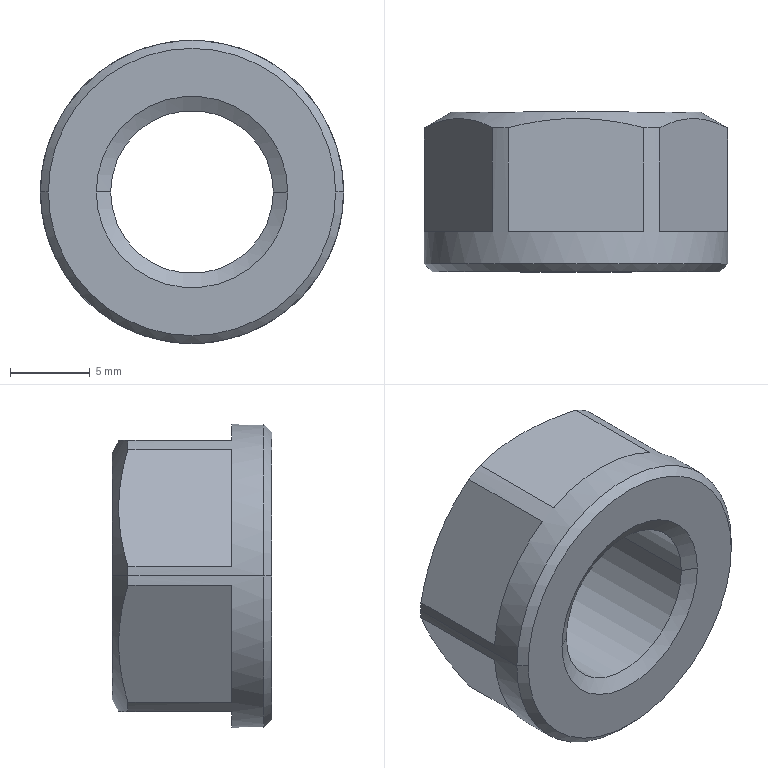Part | SolidWorks | features BaseBody 1 | 1 solid | 26 faces | box 19 x 10 x 19 mm | volume 1716 mm3 | plane 14 | cone 8 | cylinder 4 | commonest cylinder face diameters 10.2 x2 19 x2
STEP:
#1=CARTESIAN_POINT('',(59.5,178.7,-24.25));
#2=VERTEX_POINT('',#1);
#3=CARTESIAN_POINT('',(41.5,178.7,-24.25));
#4=VERTEX_POINT('',#3);
#5=CARTESIAN_POINT('',(50.5,178.7,-24.25));
#6=DIRECTION('',(0.,-1.,0.));
#7=DIRECTION('',(-1.,0.,0.));
#8=AXIS2_PLACEMENT_3D('',#5,#6,#7);
#9=CIRCLE('',#8,9.);
#10=EDGE_CURVE('',#2,#4,#9,.T.);
#11=ORIENTED_EDGE('',*,*,#10,.F.);
#12=CARTESIAN_POINT('',(60.,179.2,-24.25));
#13=VERTEX_POINT('',#12);
#14=CARTESIAN_POINT('',(60.,179.2,-24.25));
#15=DIRECTION('',(0.7071,0.7071,0.));
#16=VECTOR('',#15,1000.);
#17=LINE('',#14,#16);
#18=EDGE_CURVE('',#2,#13,#17,.T.);
#19=ORIENTED_EDGE('',*,*,#18,.T.);
#20=CARTESIAN_POINT('',(41.,179.2,-24.25));
#21=VERTEX_POINT('',#20);
#22=CARTESIAN_POINT('',(50.5,179.2,-24.25));
#23=DIRECTION('',(0.,1.,0.));
#24=DIRECTION('',(-1.,0.,0.));
#25=AXIS2_PLACEMENT_3D('',#22,#23,#24);
#26=CIRCLE('',#25,9.5);
#27=EDGE_CURVE('',#21,#13,#26,.T.);
#28=ORIENTED_EDGE('',*,*,#27,.F.);
#29=CARTESIAN_POINT('',(41.,179.2,-24.25));
#30=DIRECTION('',(-0.7071,0.7071,0.));
#31=VECTOR('',#30,1000.);
#32=LINE('',#29,#31);
#33=EDGE_CURVE('',#4,#21,#32,.T.);
#34=ORIENTED_EDGE('',*,*,#33,.F.);
#35=EDGE_LOOP('',(#11,#19,#28,#34));
#36=FACE_OUTER_BOUND('',#35,.T.);
#37=CARTESIAN_POINT('',(50.5,179.2,-24.25));
#38=DIRECTION('',(0.,1.,0.));
#39=DIRECTION('',(-1.,0.,0.));
#40=AXIS2_PLACEMENT_3D('',#37,#38,#39);
#41=CONICAL_SURFACE('',#40,9.5,0.7854);
#42=ADVANCED_FACE('',(#36),#41,.T.);
#43=CARTESIAN_POINT('',(58.294,188.7,-24.25));
#44=VERTEX_POINT('',#43);
#45=CARTESIAN_POINT('',(42.706,188.7,-24.25));
#46=VERTEX_POINT('',#45);
#47=CARTESIAN_POINT('',(50.5,188.7,-24.25));
#48=DIRECTION('',(0.,1.,0.));
#49=DIRECTION('',(-1.,0.,0.));
#50=AXIS2_PLACEMENT_3D('',#47,#48,#49);
#51=CIRCLE('',#50,7.794);
#52=EDGE_CURVE('',#44,#46,#51,.T.);
#53=ORIENTED_EDGE('',*,*,#52,.F.);
#54=CARTESIAN_POINT('',(60.,187.715,-24.25));
#55=VERTEX_POINT('',#54);
#56=CARTESIAN_POINT('',(58.294,188.7,-24.25));
#57=DIRECTION('',(0.866,-0.5,0.));
#58=VECTOR('',#57,1000.);
#59=LINE('',#56,#58);
#60=EDGE_CURVE('',#44,#55,#59,.T.);
#61=ORIENTED_EDGE('',*,*,#60,.T.);
#62=CARTESIAN_POINT('',(59.983,187.715,-24.826));
#63=VERTEX_POINT('',#62);
#64=CARTESIAN_POINT('',(50.5,187.715,-24.25));
#65=DIRECTION('',(0.,1.,0.));
#66=DIRECTION('',(1.,0.,0.));
#67=AXIS2_PLACEMENT_3D('',#64,#65,#66);
#68=CIRCLE('',#67,9.5);
#69=EDGE_CURVE('',#55,#63,#68,.T.);
#70=ORIENTED_EDGE('',*,*,#69,.T.);
#71=CARTESIAN_POINT('',(55.74,187.715,-32.174));
#72=VERTEX_POINT('',#71);
#73=CARTESIAN_POINT('',(59.983,187.715,-24.826));
#74=CARTESIAN_POINT('',(59.635,187.895,-25.428));
#75=CARTESIAN_POINT('',(59.285,188.039,-26.034));
#76=CARTESIAN_POINT('',(58.581,188.238,-27.254));
#77=CARTESIAN_POINT('',(58.226,188.292,-27.868));
#78=CARTESIAN_POINT('',(57.511,188.293,-29.106));
#79=CARTESIAN_POINT('',(57.15,188.24,-29.732));
#80=CARTESIAN_POINT('',(56.44,188.041,-30.962));
#81=CARTESIAN_POINT('',(56.088,187.895,-31.571));
#82=CARTESIAN_POINT('',(55.74,187.715,-32.174));
#83=B_SPLINE_CURVE_WITH_KNOTS('',3,(#73,#74,#75,#76,#77,#78,#79,#80,#81,#82),.UNSPECIFIED.,.F.,.F.,(4,2,2,2,4),(0.000000295,0.002133,0.004266,0.006398,0.008531),.UNSPECIFIED.);
#84=EDGE_CURVE('',#63,#72,#83,.T.);
#85=ORIENTED_EDGE('',*,*,#84,.T.);
#86=CARTESIAN_POINT('',(54.743,187.715,-32.75));
#87=VERTEX_POINT('',#86);
#88=CARTESIAN_POINT('',(50.5,187.715,-24.25));
#89=DIRECTION('',(0.,1.,0.));
#90=DIRECTION('',(1.,0.,0.));
#91=AXIS2_PLACEMENT_3D('',#88,#89,#90);
#92=CIRCLE('',#91,9.5);
#93=EDGE_CURVE('',#72,#87,#92,.T.);
#94=ORIENTED_EDGE('',*,*,#93,.T.);
#95=CARTESIAN_POINT('',(46.257,187.715,-32.75));
#96=VERTEX_POINT('',#95);
#97=CARTESIAN_POINT('',(54.743,187.715,-32.75));
#98=CARTESIAN_POINT('',(54.047,187.895,-32.75));
#99=CARTESIAN_POINT('',(53.348,188.039,-32.75));
#100=CARTESIAN_POINT('',(51.939,188.238,-32.75));
#101=CARTESIAN_POINT('',(51.23,188.292,-32.75));
#102=CARTESIAN_POINT('',(49.8,188.293,-32.75));
#103=CARTESIAN_POINT('',(49.078,188.24,-32.75));
#104=CARTESIAN_POINT('',(47.657,188.041,-32.75));
#105=CARTESIAN_POINT('',(46.954,187.895,-32.75));
#106=CARTESIAN_POINT('',(46.257,187.715,-32.75));
#107=B_SPLINE_CURVE_WITH_KNOTS('',3,(#97,#98,#99,#100,#101,#102,#103,#104,#105,#106),.UNSPECIFIED.,.F.,.F.,(4,2,2,2,4),(0.000000255,0.002133,0.004266,0.006398,0.008531),.UNSPECIFIED.);
#108=EDGE_CURVE('',#87,#96,#107,.T.);
#109=ORIENTED_EDGE('',*,*,#108,.T.);
#110=CARTESIAN_POINT('',(45.26,187.715,-32.174));
#111=VERTEX_POINT('',#110);
#112=CARTESIAN_POINT('',(50.5,187.715,-24.25));
#113=DIRECTION('',(0.,1.,0.));
#114=DIRECTION('',(1.,0.,0.));
#115=AXIS2_PLACEMENT_3D('',#112,#113,#114);
#116=CIRCLE('',#115,9.5);
#117=EDGE_CURVE('',#96,#111,#116,.T.);
#118=ORIENTED_EDGE('',*,*,#117,.T.);
#119=CARTESIAN_POINT('',(41.017,187.715,-24.826));
#120=VERTEX_POINT('',#119);
#121=CARTESIAN_POINT('',(45.26,187.715,-32.174));
#122=CARTESIAN_POINT('',(44.912,187.895,-31.572));
#123=CARTESIAN_POINT('',(44.563,188.039,-30.966));
#124=CARTESIAN_POINT('',(43.858,188.238,-29.746));
#125=CARTESIAN_POINT('',(43.504,188.292,-29.132));
#126=CARTESIAN_POINT('',(42.789,188.293,-27.894));
#127=CARTESIAN_POINT('',(42.428,188.24,-27.268));
#128=CARTESIAN_POINT('',(41.717,188.041,-26.038));
#129=CARTESIAN_POINT('',(41.366,187.895,-25.429));
#130=CARTESIAN_POINT('',(41.017,187.715,-24.826));
#131=B_SPLINE_CURVE_WITH_KNOTS('',3,(#121,#122,#123,#124,#125,#126,#127,#128,#129,#130),.UNSPECIFIED.,.F.,.F.,(4,2,2,2,4),(0.000000295,0.002133,0.004266,0.006398,0.008531),.UNSPECIFIED.);
#132=EDGE_CURVE('',#111,#120,#131,.T.);
#133=ORIENTED_EDGE('',*,*,#132,.T.);
#134=CARTESIAN_POINT('',(41.,187.715,-24.25));
#135=VERTEX_POINT('',#134);
#136=CARTESIAN_POINT('',(50.5,187.715,-24.25));
#137=DIRECTION('',(0.,1.,0.));
#138=DIRECTION('',(1.,0.,0.));
#139=AXIS2_PLACEMENT_3D('',#136,#137,#138);
#140=CIRCLE('',#139,9.5);
#141=EDGE_CURVE('',#120,#135,#140,.T.);
#142=ORIENTED_EDGE('',*,*,#141,.T.);
#143=CARTESIAN_POINT('',(42.706,188.7,-24.25));
#144=DIRECTION('',(-0.866,-0.5,0.));
#145=VECTOR('',#144,1000.);
#146=LINE('',#143,#145);
#147=EDGE_CURVE('',#46,#135,#146,.T.);
#148=ORIENTED_EDGE('',*,*,#147,.F.);
#149=EDGE_LOOP('',(#53,#61,#70,#85,#94,#109,#118,#133,#142,#148));
#150=FACE_OUTER_BOUND('',#149,.T.);
#151=CARTESIAN_POINT('',(50.5,188.7,-24.25));
#152=DIRECTION('',(0.,-1.,0.));
#153=DIRECTION('',(-1.,0.,0.));
#154=AXIS2_PLACEMENT_3D('',#151,#152,#153);
#155=CONICAL_SURFACE('',#154,7.794,1.047);
#156=ADVANCED_FACE('',(#150),#155,.T.);
#157=CARTESIAN_POINT('',(55.6,179.22,-24.25));
#158=VERTEX_POINT('',#157);
#159=CARTESIAN_POINT('',(45.4,179.22,-24.25));
#160=VERTEX_POINT('',#159);
#161=CARTESIAN_POINT('',(50.5,179.22,-24.25));
#162=DIRECTION('',(0.,1.,0.));
#163=DIRECTION('',(-1.,0.,0.));
#164=AXIS2_PLACEMENT_3D('',#161,#162,#163);
#165=CIRCLE('',#164,5.1);
#166=EDGE_CURVE('',#158,#160,#165,.T.);
#167=ORIENTED_EDGE('',*,*,#166,.T.);
#168=CARTESIAN_POINT('',(44.5,178.7,-24.25));
#169=VERTEX_POINT('',#168);
#170=CARTESIAN_POINT('',(45.4,179.22,-24.25));
#171=DIRECTION('',(-0.866,-0.5,0.));
#172=VECTOR('',#171,1000.);
#173=LINE('',#170,#172);
#174=EDGE_CURVE('',#160,#169,#173,.T.);
#175=ORIENTED_EDGE('',*,*,#174,.T.);
#176=CARTESIAN_POINT('',(56.5,178.7,-24.25));
#177=VERTEX_POINT('',#176);
#178=CARTESIAN_POINT('',(50.5,178.7,-24.25));
#179=DIRECTION('',(0.,1.,0.));
#180=DIRECTION('',(-1.,0.,0.));
#181=AXIS2_PLACEMENT_3D('',#178,#179,#180);
#182=CIRCLE('',#181,6.);
#183=EDGE_CURVE('',#177,#169,#182,.T.);
#184=ORIENTED_EDGE('',*,*,#183,.F.);
#185=CARTESIAN_POINT('',(55.6,179.22,-24.25));
#186=DIRECTION('',(0.866,-0.5,0.));
#187=VECTOR('',#186,1000.);
#188=LINE('',#185,#187);
#189=EDGE_CURVE('',#158,#177,#188,.T.);
#190=ORIENTED_EDGE('',*,*,#189,.F.);
#191=EDGE_LOOP('',(#167,#175,#184,#190));
#192=FACE_OUTER_BOUND('',#191,.T.);
#193=CARTESIAN_POINT('',(50.5,179.22,-24.25));
#194=DIRECTION('',(0.,-1.,0.));
#195=DIRECTION('',(1.,0.,0.));
#196=AXIS2_PLACEMENT_3D('',#193,#194,#195);
#197=CONICAL_SURFACE('',#196,5.1,1.047);
#198=ADVANCED_FACE('',(#192),#197,.F.);
#199=ORIENTED_EDGE('',*,*,#166,.F.);
#200=CARTESIAN_POINT('',(55.6,188.18,-24.25));
#201=VERTEX_POINT('',#200);
#202=CARTESIAN_POINT('',(55.6,188.7,-24.25));
#203=DIRECTION('',(0.,1.,0.));
#204=VECTOR('',#203,1000.);
#205=LINE('',#202,#204);
#206=EDGE_CURVE('',#158,#201,#205,.T.);
#207=ORIENTED_EDGE('',*,*,#206,.T.);
#208=CARTESIAN_POINT('',(45.4,188.18,-24.25));
#209=VERTEX_POINT('',#208);
#210=CARTESIAN_POINT('',(50.5,188.18,-24.25));
#211=DIRECTION('',(0.,1.,0.));
#212=DIRECTION('',(-1.,0.,0.));
#213=AXIS2_PLACEMENT_3D('',#210,#211,#212);
#214=CIRCLE('',#213,5.1);
#215=EDGE_CURVE('',#201,#209,#214,.T.);
#216=ORIENTED_EDGE('',*,*,#215,.T.);
#217=CARTESIAN_POINT('',(45.4,188.7,-24.25));
#218=DIRECTION('',(0.,1.,0.));
#219=VECTOR('',#218,1000.);
#220=LINE('',#217,#219);
#221=EDGE_CURVE('',#160,#209,#220,.T.);
#222=ORIENTED_EDGE('',*,*,#221,.F.);
#223=EDGE_LOOP('',(#199,#207,#216,#222));
#224=FACE_OUTER_BOUND('',#223,.T.);
#225=CARTESIAN_POINT('',(50.5,188.7,-24.25));
#226=DIRECTION('',(0.,1.,0.));
#227=DIRECTION('',(-1.,0.,0.));
#228=AXIS2_PLACEMENT_3D('',#225,#226,#227);
#229=CYLINDRICAL_SURFACE('',#228,5.1);
#230=ADVANCED_FACE('',(#224),#229,.F.);
#231=ORIENTED_EDGE('',*,*,#215,.F.);
#232=CARTESIAN_POINT('',(56.5,188.7,-24.25));
#233=VERTEX_POINT('',#232);
#234=CARTESIAN_POINT('',(56.5,188.7,-24.25));
#235=DIRECTION('',(0.866,0.5,0.));
#236=VECTOR('',#235,1000.);
#237=LINE('',#234,#236);
#238=EDGE_CURVE('',#201,#233,#237,.T.);
#239=ORIENTED_EDGE('',*,*,#238,.T.);
#240=CARTESIAN_POINT('',(44.5,188.7,-24.25));
#241=VERTEX_POINT('',#240);
#242=CARTESIAN_POINT('',(50.5,188.7,-24.25));
#243=DIRECTION('',(0.,1.,0.));
#244=DIRECTION('',(-1.,0.,0.));
#245=AXIS2_PLACEMENT_3D('',#242,#243,#244);
#246=CIRCLE('',#245,6.);
#247=EDGE_CURVE('',#233,#241,#246,.T.);
#248=ORIENTED_EDGE('',*,*,#247,.T.);
#249=CARTESIAN_POINT('',(44.5,188.7,-24.25));
#250=DIRECTION('',(-0.866,0.5,0.));
#251=VECTOR('',#250,1000.);
#252=LINE('',#249,#251);
#253=EDGE_CURVE('',#209,#241,#252,.T.);
#254=ORIENTED_EDGE('',*,*,#253,.F.);
#255=EDGE_LOOP('',(#231,#239,#248,#254));
#256=FACE_OUTER_BOUND('',#255,.T.);
#257=CARTESIAN_POINT('',(50.5,188.7,-24.25));
#258=DIRECTION('',(0.,1.,0.));
#259=DIRECTION('',(-1.,0.,0.));
#260=AXIS2_PLACEMENT_3D('',#257,#258,#259);
#261=CONICAL_SURFACE('',#260,6.,1.047);
#262=ADVANCED_FACE('',(#256),#261,.F.);
#263=CARTESIAN_POINT('',(41.017,187.715,-23.674));
#264=VERTEX_POINT('',#263);
#265=CARTESIAN_POINT('',(50.5,187.715,-24.25));
#266=DIRECTION('',(0.,1.,0.));
#267=DIRECTION('',(1.,0.,0.));
#268=AXIS2_PLACEMENT_3D('',#265,#266,#267);
#269=CIRCLE('',#268,9.5);
#270=EDGE_CURVE('',#135,#264,#269,.T.);
#271=ORIENTED_EDGE('',*,*,#270,.F.);
#272=CARTESIAN_POINT('',(41.,181.2,-24.25));
#273=DIRECTION('',(0.,-1.,0.));
#274=VECTOR('',#273,1000.);
#275=LINE('',#272,#274);
#276=EDGE_CURVE('',#135,#21,#275,.T.);
#277=ORIENTED_EDGE('',*,*,#276,.T.);
#278=ORIENTED_EDGE('',*,*,#27,.T.);
#279=CARTESIAN_POINT('',(60.,181.2,-24.25));
#280=DIRECTION('',(0.,-1.,0.));
#281=VECTOR('',#280,1000.);
#282=LINE('',#279,#281);
#283=EDGE_CURVE('',#55,#13,#282,.T.);
#284=ORIENTED_EDGE('',*,*,#283,.F.);
#285=CARTESIAN_POINT('',(59.983,187.715,-23.674));
#286=VERTEX_POINT('',#285);
#287=CARTESIAN_POINT('',(50.5,187.715,-24.25));
#288=DIRECTION('',(0.,1.,0.));
#289=DIRECTION('',(1.,0.,0.));
#290=AXIS2_PLACEMENT_3D('',#287,#288,#289);
#291=CIRCLE('',#290,9.5);
#292=EDGE_CURVE('',#286,#55,#291,.T.);
#293=ORIENTED_EDGE('',*,*,#292,.F.);
#294=CARTESIAN_POINT('',(59.983,181.2,-23.674));
#295=VERTEX_POINT('',#294);
#296=CARTESIAN_POINT('',(59.983,224.195,-23.674));
#297=DIRECTION('',(0.,-1.,0.));
#298=VECTOR('',#297,1000.);
#299=LINE('',#296,#298);
#300=EDGE_CURVE('',#286,#295,#299,.T.);
#301=ORIENTED_EDGE('',*,*,#300,.T.);
#302=CARTESIAN_POINT('',(55.74,181.2,-16.326));
#303=VERTEX_POINT('',#302);
#304=CARTESIAN_POINT('',(50.5,181.2,-24.25));
#305=DIRECTION('',(0.,1.,0.));
#306=DIRECTION('',(-1.,0.,0.));
#307=AXIS2_PLACEMENT_3D('',#304,#305,#306);
#308=CIRCLE('',#307,9.5);
#309=EDGE_CURVE('',#303,#295,#308,.T.);
#310=ORIENTED_EDGE('',*,*,#309,.F.);
#311=CARTESIAN_POINT('',(55.74,187.715,-16.326));
#312=VERTEX_POINT('',#311);
#313=CARTESIAN_POINT('',(55.74,224.195,-16.326));
#314=DIRECTION('',(0.,-1.,0.));
#315=VECTOR('',#314,1000.);
#316=LINE('',#313,#315);
#317=EDGE_CURVE('',#312,#303,#316,.T.);
#318=ORIENTED_EDGE('',*,*,#317,.F.);
#319=CARTESIAN_POINT('',(54.743,187.715,-15.75));
#320=VERTEX_POINT('',#319);
#321=CARTESIAN_POINT('',(50.5,187.715,-24.25));
#322=DIRECTION('',(0.,1.,0.));
#323=DIRECTION('',(1.,0.,0.));
#324=AXIS2_PLACEMENT_3D('',#321,#322,#323);
#325=CIRCLE('',#324,9.5);
#326=EDGE_CURVE('',#320,#312,#325,.T.);
#327=ORIENTED_EDGE('',*,*,#326,.F.);
#328=CARTESIAN_POINT('',(54.743,181.2,-15.75));
#329=VERTEX_POINT('',#328);
#330=CARTESIAN_POINT('',(54.743,224.195,-15.75));
#331=DIRECTION('',(0.,-1.,0.));
#332=VECTOR('',#331,1000.);
#333=LINE('',#330,#332);
#334=EDGE_CURVE('',#320,#329,#333,.T.);
#335=ORIENTED_EDGE('',*,*,#334,.T.);
#336=CARTESIAN_POINT('',(46.257,181.2,-15.75));
#337=VERTEX_POINT('',#336);
#338=CARTESIAN_POINT('',(50.5,181.2,-24.25));
#339=DIRECTION('',(0.,1.,0.));
#340=DIRECTION('',(-1.,0.,0.));
#341=AXIS2_PLACEMENT_3D('',#338,#339,#340);
#342=CIRCLE('',#341,9.5);
#343=EDGE_CURVE('',#337,#329,#342,.T.);
#344=ORIENTED_EDGE('',*,*,#343,.F.);
#345=CARTESIAN_POINT('',(46.257,187.715,-15.75));
#346=VERTEX_POINT('',#345);
#347=CARTESIAN_POINT('',(46.257,224.195,-15.75));
#348=DIRECTION('',(0.,-1.,0.));
#349=VECTOR('',#348,1000.);
#350=LINE('',#347,#349);
#351=EDGE_CURVE('',#346,#337,#350,.T.);
#352=ORIENTED_EDGE('',*,*,#351,.F.);
#353=CARTESIAN_POINT('',(45.26,187.715,-16.326));
#354=VERTEX_POINT('',#353);
#355=CARTESIAN_POINT('',(50.5,187.715,-24.25));
#356=DIRECTION('',(0.,1.,0.));
#357=DIRECTION('',(1.,0.,0.));
#358=AXIS2_PLACEMENT_3D('',#355,#356,#357);
#359=CIRCLE('',#358,9.5);
#360=EDGE_CURVE('',#354,#346,#359,.T.);
#361=ORIENTED_EDGE('',*,*,#360,.F.);
#362=CARTESIAN_POINT('',(45.26,181.2,-16.326));
#363=VERTEX_POINT('',#362);
#364=CARTESIAN_POINT('',(45.26,224.195,-16.326));
#365=DIRECTION('',(0.,-1.,0.));
#366=VECTOR('',#365,1000.);
#367=LINE('',#364,#366);
#368=EDGE_CURVE('',#354,#363,#367,.T.);
#369=ORIENTED_EDGE('',*,*,#368,.T.);
#370=CARTESIAN_POINT('',(41.017,181.2,-23.674));
#371=VERTEX_POINT('',#370);
#372=CARTESIAN_POINT('',(50.5,181.2,-24.25));
#373=DIRECTION('',(0.,1.,0.));
#374=DIRECTION('',(-1.,0.,0.));
#375=AXIS2_PLACEMENT_3D('',#372,#373,#374);
#376=CIRCLE('',#375,9.5);
#377=EDGE_CURVE('',#371,#363,#376,.T.);
#378=ORIENTED_EDGE('',*,*,#377,.F.);
#379=CARTESIAN_POINT('',(41.017,224.195,-23.674));
#380=DIRECTION('',(0.,-1.,0.));
#381=VECTOR('',#380,1000.);
#382=LINE('',#379,#381);
#383=EDGE_CURVE('',#264,#371,#382,.T.);
#384=ORIENTED_EDGE('',*,*,#383,.F.);
#385=EDGE_LOOP('',(#271,#277,#278,#284,#293,#301,#310,#318,#327,#335,#344,#352,#361,#369,#378,#384));
#386=FACE_OUTER_BOUND('',#385,.T.);
#387=CARTESIAN_POINT('',(50.5,181.2,-24.25));
#388=DIRECTION('',(0.,-1.,0.));
#389=DIRECTION('',(1.,0.,0.));
#390=AXIS2_PLACEMENT_3D('',#387,#388,#389);
#391=CYLINDRICAL_SURFACE('',#390,9.5);
#392=ADVANCED_FACE('',(#386),#391,.T.);
#393=ORIENTED_EDGE('',*,*,#276,.F.);
#394=ORIENTED_EDGE('',*,*,#141,.F.);
#395=CARTESIAN_POINT('',(41.017,181.2,-24.826));
#396=VERTEX_POINT('',#395);
#397=CARTESIAN_POINT('',(41.017,224.195,-24.826));
#398=DIRECTION('',(0.,-1.,0.));
#399=VECTOR('',#398,1000.);
#400=LINE('',#397,#399);
#401=EDGE_CURVE('',#120,#396,#400,.T.);
#402=ORIENTED_EDGE('',*,*,#401,.T.);
#403=CARTESIAN_POINT('',(45.26,181.2,-32.174));
#404=VERTEX_POINT('',#403);
#405=CARTESIAN_POINT('',(50.5,181.2,-24.25));
#406=DIRECTION('',(0.,1.,0.));
#407=DIRECTION('',(-1.,0.,0.));
#408=AXIS2_PLACEMENT_3D('',#405,#406,#407);
#409=CIRCLE('',#408,9.5);
#410=EDGE_CURVE('',#404,#396,#409,.T.);
#411=ORIENTED_EDGE('',*,*,#410,.F.);
#412=CARTESIAN_POINT('',(45.26,224.195,-32.174));
#413=DIRECTION('',(0.,-1.,0.));
#414=VECTOR('',#413,1000.);
#415=LINE('',#412,#414);
#416=EDGE_CURVE('',#111,#404,#415,.T.);
#417=ORIENTED_EDGE('',*,*,#416,.F.);
#418=ORIENTED_EDGE('',*,*,#117,.F.);
#419=CARTESIAN_POINT('',(46.257,181.2,-32.75));
#420=VERTEX_POINT('',#419);
#421=CARTESIAN_POINT('',(46.257,224.195,-32.75));
#422=DIRECTION('',(0.,-1.,0.));
#423=VECTOR('',#422,1000.);
#424=LINE('',#421,#423);
#425=EDGE_CURVE('',#96,#420,#424,.T.);
#426=ORIENTED_EDGE('',*,*,#425,.T.);
#427=CARTESIAN_POINT('',(54.743,181.2,-32.75));
#428=VERTEX_POINT('',#427);
#429=CARTESIAN_POINT('',(50.5,181.2,-24.25));
#430=DIRECTION('',(0.,1.,0.));
#431=DIRECTION('',(-1.,0.,0.));
#432=AXIS2_PLACEMENT_3D('',#429,#430,#431);
#433=CIRCLE('',#432,9.5);
#434=EDGE_CURVE('',#428,#420,#433,.T.);
#435=ORIENTED_EDGE('',*,*,#434,.F.);
#436=CARTESIAN_POINT('',(54.743,224.195,-32.75));
#437=DIRECTION('',(0.,-1.,0.));
#438=VECTOR('',#437,1000.);
#439=LINE('',#436,#438);
#440=EDGE_CURVE('',#87,#428,#439,.T.);
#441=ORIENTED_EDGE('',*,*,#440,.F.);
#442=ORIENTED_EDGE('',*,*,#93,.F.);
#443=CARTESIAN_POINT('',(55.74,181.2,-32.174));
#444=VERTEX_POINT('',#443);
#445=CARTESIAN_POINT('',(55.74,224.195,-32.174));
#446=DIRECTION('',(0.,-1.,0.));
#447=VECTOR('',#446,1000.);
#448=LINE('',#445,#447);
#449=EDGE_CURVE('',#72,#444,#448,.T.);
#450=ORIENTED_EDGE('',*,*,#449,.T.);
#451=CARTESIAN_POINT('',(59.983,181.2,-24.826));
#452=VERTEX_POINT('',#451);
#453=CARTESIAN_POINT('',(50.5,181.2,-24.25));
#454=DIRECTION('',(0.,1.,0.));
#455=DIRECTION('',(-1.,0.,0.));
#456=AXIS2_PLACEMENT_3D('',#453,#454,#455);
#457=CIRCLE('',#456,9.5);
#458=EDGE_CURVE('',#452,#444,#457,.T.);
#459=ORIENTED_EDGE('',*,*,#458,.F.);
#460=CARTESIAN_POINT('',(59.983,224.195,-24.826));
#461=DIRECTION('',(0.,-1.,0.));
#462=VECTOR('',#461,1000.);
#463=LINE('',#460,#462);
#464=EDGE_CURVE('',#63,#452,#463,.T.);
#465=ORIENTED_EDGE('',*,*,#464,.F.);
#466=ORIENTED_EDGE('',*,*,#69,.F.);
#467=ORIENTED_EDGE('',*,*,#283,.T.);
#468=CARTESIAN_POINT('',(50.5,179.2,-24.25));
#469=DIRECTION('',(0.,1.,0.));
#470=DIRECTION('',(-1.,0.,0.));
#471=AXIS2_PLACEMENT_3D('',#468,#469,#470);
#472=CIRCLE('',#471,9.5);
#473=EDGE_CURVE('',#13,#21,#472,.T.);
#474=ORIENTED_EDGE('',*,*,#473,.T.);
#475=EDGE_LOOP('',(#393,#394,#402,#411,#417,#418,#426,#435,#441,#442,#450,#459,#465,#466,#467,#474));
#476=FACE_OUTER_BOUND('',#475,.T.);
#477=CARTESIAN_POINT('',(50.5,181.2,-24.25));
#478=DIRECTION('',(0.,-1.,0.));
#479=DIRECTION('',(1.,0.,0.));
#480=AXIS2_PLACEMENT_3D('',#477,#478,#479);
#481=CYLINDRICAL_SURFACE('',#480,9.5);
#482=ADVANCED_FACE('',(#476),#481,.T.);
#483=CARTESIAN_POINT('',(46.257,187.715,-15.75));
#484=CARTESIAN_POINT('',(46.953,187.895,-15.75));
#485=CARTESIAN_POINT('',(47.652,188.039,-15.75));
#486=CARTESIAN_POINT('',(49.061,188.238,-15.75));
#487=CARTESIAN_POINT('',(49.77,188.292,-15.75));
#488=CARTESIAN_POINT('',(51.2,188.293,-15.75));
#489=CARTESIAN_POINT('',(51.922,188.24,-15.75));
#490=CARTESIAN_POINT('',(53.343,188.041,-15.75));
#491=CARTESIAN_POINT('',(54.046,187.895,-15.75));
#492=CARTESIAN_POINT('',(54.743,187.715,-15.75));
#493=B_SPLINE_CURVE_WITH_KNOTS('',3,(#483,#484,#485,#486,#487,#488,#489,#490,#491,#492),.UNSPECIFIED.,.F.,.F.,(4,2,2,2,4),(0.000000255,0.002133,0.004266,0.006398,0.008531),.UNSPECIFIED.);
#494=EDGE_CURVE('',#346,#320,#493,.T.);
#495=ORIENTED_EDGE('',*,*,#494,.F.);
#496=ORIENTED_EDGE('',*,*,#351,.T.);
#497=CARTESIAN_POINT('',(46.257,181.2,-15.75));
#498=DIRECTION('',(1.,0.,0.));
#499=VECTOR('',#498,1000.);
#500=LINE('',#497,#499);
#501=EDGE_CURVE('',#337,#329,#500,.T.);
#502=ORIENTED_EDGE('',*,*,#501,.T.);
#503=ORIENTED_EDGE('',*,*,#334,.F.);
#504=EDGE_LOOP('',(#495,#496,#502,#503));
#505=FACE_OUTER_BOUND('',#504,.T.);
#506=CARTESIAN_POINT('',(46.257,224.195,-15.75));
#507=DIRECTION('',(0.,0.,-1.));
#508=DIRECTION('',(0.,-1.,0.));
#509=AXIS2_PLACEMENT_3D('',#506,#507,#508);
#510=PLANE('',#509);
#511=ADVANCED_FACE('',(#505),#510,.F.);
#512=CARTESIAN_POINT('',(55.74,187.715,-16.326));
#513=CARTESIAN_POINT('',(56.088,187.895,-16.928));
#514=CARTESIAN_POINT('',(56.437,188.039,-17.534));
#515=CARTESIAN_POINT('',(57.142,188.238,-18.754));
#516=CARTESIAN_POINT('',(57.496,188.292,-19.368));
#517=CARTESIAN_POINT('',(58.211,188.293,-20.606));
#518=CARTESIAN_POINT('',(58.572,188.24,-21.232));
#519=CARTESIAN_POINT('',(59.283,188.041,-22.462));
#520=CARTESIAN_POINT('',(59.634,187.895,-23.071));
#521=CARTESIAN_POINT('',(59.983,187.715,-23.674));
#522=B_SPLINE_CURVE_WITH_KNOTS('',3,(#512,#513,#514,#515,#516,#517,#518,#519,#520,#521),.UNSPECIFIED.,.F.,.F.,(4,2,2,2,4),(0.000000295,0.002133,0.004266,0.006398,0.008531),.UNSPECIFIED.);
#523=EDGE_CURVE('',#312,#286,#522,.T.);
#524=ORIENTED_EDGE('',*,*,#523,.F.);
#525=ORIENTED_EDGE('',*,*,#317,.T.);
#526=CARTESIAN_POINT('',(55.74,181.2,-16.326));
#527=DIRECTION('',(0.5,0.,-0.866));
#528=VECTOR('',#527,1000.);
#529=LINE('',#526,#528);
#530=EDGE_CURVE('',#303,#295,#529,.T.);
#531=ORIENTED_EDGE('',*,*,#530,.T.);
#532=ORIENTED_EDGE('',*,*,#300,.F.);
#533=EDGE_LOOP('',(#524,#525,#531,#532));
#534=FACE_OUTER_BOUND('',#533,.T.);
#535=CARTESIAN_POINT('',(55.74,224.195,-16.326));
#536=DIRECTION('',(-0.866,0.,-0.5));
#537=DIRECTION('',(-0.5,0.,0.866));
#538=AXIS2_PLACEMENT_3D('',#535,#536,#537);
#539=PLANE('',#538);
#540=ADVANCED_FACE('',(#534),#539,.F.);
#541=ORIENTED_EDGE('',*,*,#84,.F.);
#542=ORIENTED_EDGE('',*,*,#464,.T.);
#543=CARTESIAN_POINT('',(59.983,181.2,-24.826));
#544=DIRECTION('',(-0.5,0.,-0.866));
#545=VECTOR('',#544,1000.);
#546=LINE('',#543,#545);
#547=EDGE_CURVE('',#452,#444,#546,.T.);
#548=ORIENTED_EDGE('',*,*,#547,.T.);
#549=ORIENTED_EDGE('',*,*,#449,.F.);
#550=EDGE_LOOP('',(#541,#542,#548,#549));
#551=FACE_OUTER_BOUND('',#550,.T.);
#552=CARTESIAN_POINT('',(59.983,224.195,-24.826));
#553=DIRECTION('',(-0.866,0.,0.5));
#554=DIRECTION('',(0.5,0.,0.866));
#555=AXIS2_PLACEMENT_3D('',#552,#553,#554);
#556=PLANE('',#555);
#557=ADVANCED_FACE('',(#551),#556,.F.);
#558=ORIENTED_EDGE('',*,*,#108,.F.);
#559=ORIENTED_EDGE('',*,*,#440,.T.);
#560=CARTESIAN_POINT('',(54.743,181.2,-32.75));
#561=DIRECTION('',(-1.,0.,0.));
#562=VECTOR('',#561,1000.);
#563=LINE('',#560,#562);
#564=EDGE_CURVE('',#428,#420,#563,.T.);
#565=ORIENTED_EDGE('',*,*,#564,.T.);
#566=ORIENTED_EDGE('',*,*,#425,.F.);
#567=EDGE_LOOP('',(#558,#559,#565,#566));
#568=FACE_OUTER_BOUND('',#567,.T.);
#569=CARTESIAN_POINT('',(54.743,224.195,-32.75));
#570=DIRECTION('',(0.,0.,1.));
#571=DIRECTION('',(0.,1.,0.));
#572=AXIS2_PLACEMENT_3D('',#569,#570,#571);
#573=PLANE('',#572);
#574=ADVANCED_FACE('',(#568),#573,.F.);
#575=ORIENTED_EDGE('',*,*,#132,.F.);
#576=ORIENTED_EDGE('',*,*,#416,.T.);
#577=CARTESIAN_POINT('',(45.26,181.2,-32.174));
#578=DIRECTION('',(-0.5,0.,0.866));
#579=VECTOR('',#578,1000.);
#580=LINE('',#577,#579);
#581=EDGE_CURVE('',#404,#396,#580,.T.);
#582=ORIENTED_EDGE('',*,*,#581,.T.);
#583=ORIENTED_EDGE('',*,*,#401,.F.);
#584=EDGE_LOOP('',(#575,#576,#582,#583));
#585=FACE_OUTER_BOUND('',#584,.T.);
#586=CARTESIAN_POINT('',(45.26,224.195,-32.174));
#587=DIRECTION('',(0.866,0.,0.5));
#588=DIRECTION('',(0.5,0.,-0.866));
#589=AXIS2_PLACEMENT_3D('',#586,#587,#588);
#590=PLANE('',#589);
#591=ADVANCED_FACE('',(#585),#590,.F.);
#592=CARTESIAN_POINT('',(41.017,187.715,-23.674));
#593=CARTESIAN_POINT('',(41.365,187.895,-23.072));
#594=CARTESIAN_POINT('',(41.715,188.039,-22.466));
#595=CARTESIAN_POINT('',(42.419,188.238,-21.246));
#596=CARTESIAN_POINT('',(42.774,188.292,-20.632));
#597=CARTESIAN_POINT('',(43.489,188.293,-19.394));
#598=CARTESIAN_POINT('',(43.85,188.24,-18.768));
#599=CARTESIAN_POINT('',(44.56,188.041,-17.538));
#600=CARTESIAN_POINT('',(44.912,187.895,-16.929));
#601=CARTESIAN_POINT('',(45.26,187.715,-16.326));
#602=B_SPLINE_CURVE_WITH_KNOTS('',3,(#592,#593,#594,#595,#596,#597,#598,#599,#600,#601),.UNSPECIFIED.,.F.,.F.,(4,2,2,2,4),(0.000000295,0.002133,0.004266,0.006398,0.008531),.UNSPECIFIED.);
#603=EDGE_CURVE('',#264,#354,#602,.T.);
#604=ORIENTED_EDGE('',*,*,#603,.F.);
#605=ORIENTED_EDGE('',*,*,#383,.T.);
#606=CARTESIAN_POINT('',(41.017,181.2,-23.674));
#607=DIRECTION('',(0.5,0.,0.866));
#608=VECTOR('',#607,1000.);
#609=LINE('',#606,#608);
#610=EDGE_CURVE('',#371,#363,#609,.T.);
#611=ORIENTED_EDGE('',*,*,#610,.T.);
#612=ORIENTED_EDGE('',*,*,#368,.F.);
#613=EDGE_LOOP('',(#604,#605,#611,#612));
#614=FACE_OUTER_BOUND('',#613,.T.);
#615=CARTESIAN_POINT('',(41.017,224.195,-23.674));
#616=DIRECTION('',(0.866,0.,-0.5));
#617=DIRECTION('',(-0.5,0.,-0.866));
#618=AXIS2_PLACEMENT_3D('',#615,#616,#617);
#619=PLANE('',#618);
#620=ADVANCED_FACE('',(#614),#619,.F.);
#621=CARTESIAN_POINT('',(50.5,188.7,-24.25));
#622=DIRECTION('',(0.,1.,0.));
#623=DIRECTION('',(-1.,0.,0.));
#624=AXIS2_PLACEMENT_3D('',#621,#622,#623);
#625=CIRCLE('',#624,6.);
#626=EDGE_CURVE('',#241,#233,#625,.T.);
#627=ORIENTED_EDGE('',*,*,#626,.F.);
#628=ORIENTED_EDGE('',*,*,#247,.F.);
#629=EDGE_LOOP('',(#627,#628));
#630=FACE_BOUND('',#629,.T.);
#631=CARTESIAN_POINT('',(50.5,188.7,-24.25));
#632=DIRECTION('',(0.,1.,0.));
#633=DIRECTION('',(-1.,0.,0.));
#634=AXIS2_PLACEMENT_3D('',#631,#632,#633);
#635=CIRCLE('',#634,7.794);
#636=EDGE_CURVE('',#46,#44,#635,.T.);
#637=ORIENTED_EDGE('',*,*,#636,.T.);
#638=ORIENTED_EDGE('',*,*,#52,.T.);
#639=EDGE_LOOP('',(#637,#638));
#640=FACE_OUTER_BOUND('',#639,.T.);
#641=CARTESIAN_POINT('',(50.5,188.7,-24.25));
#642=DIRECTION('',(0.,1.,0.));
#643=DIRECTION('',(-1.,0.,0.));
#644=AXIS2_PLACEMENT_3D('',#641,#642,#643);
#645=PLANE('',#644);
#646=ADVANCED_FACE('',(#630,#640),#645,.T.);
#647=ORIENTED_EDGE('',*,*,#610,.F.);
#648=ORIENTED_EDGE('',*,*,#377,.T.);
#649=EDGE_LOOP('',(#647,#648));
#650=FACE_OUTER_BOUND('',#649,.T.);
#651=CARTESIAN_POINT('',(50.5,181.2,-24.25));
#652=DIRECTION('',(0.,1.,0.));
#653=DIRECTION('',(-1.,0.,0.));
#654=AXIS2_PLACEMENT_3D('',#651,#652,#653);
#655=PLANE('',#654);
#656=ADVANCED_FACE('',(#650),#655,.T.);
#657=ORIENTED_EDGE('',*,*,#581,.F.);
#658=ORIENTED_EDGE('',*,*,#410,.T.);
#659=EDGE_LOOP('',(#657,#658));
#660=FACE_OUTER_BOUND('',#659,.T.);
#661=CARTESIAN_POINT('',(50.5,181.2,-24.25));
#662=DIRECTION('',(0.,1.,0.));
#663=DIRECTION('',(-1.,0.,0.));
#664=AXIS2_PLACEMENT_3D('',#661,#662,#663);
#665=PLANE('',#664);
#666=ADVANCED_FACE('',(#660),#665,.T.);
#667=ORIENTED_EDGE('',*,*,#564,.F.);
#668=ORIENTED_EDGE('',*,*,#434,.T.);
#669=EDGE_LOOP('',(#667,#668));
#670=FACE_OUTER_BOUND('',#669,.T.);
#671=CARTESIAN_POINT('',(50.5,181.2,-24.25));
#672=DIRECTION('',(0.,1.,0.));
#673=DIRECTION('',(-1.,0.,0.));
#674=AXIS2_PLACEMENT_3D('',#671,#672,#673);
#675=PLANE('',#674);
#676=ADVANCED_FACE('',(#670),#675,.T.);
#677=ORIENTED_EDGE('',*,*,#547,.F.);
#678=ORIENTED_EDGE('',*,*,#458,.T.);
#679=EDGE_LOOP('',(#677,#678));
#680=FACE_OUTER_BOUND('',#679,.T.);
#681=CARTESIAN_POINT('',(50.5,181.2,-24.25));
#682=DIRECTION('',(0.,1.,0.));
#683=DIRECTION('',(-1.,0.,0.));
#684=AXIS2_PLACEMENT_3D('',#681,#682,#683);
#685=PLANE('',#684);
#686=ADVANCED_FACE('',(#680),#685,.T.);
#687=ORIENTED_EDGE('',*,*,#530,.F.);
#688=ORIENTED_EDGE('',*,*,#309,.T.);
#689=EDGE_LOOP('',(#687,#688));
#690=FACE_OUTER_BOUND('',#689,.T.);
#691=CARTESIAN_POINT('',(50.5,181.2,-24.25));
#692=DIRECTION('',(0.,1.,0.));
#693=DIRECTION('',(-1.,0.,0.));
#694=AXIS2_PLACEMENT_3D('',#691,#692,#693);
#695=PLANE('',#694);
#696=ADVANCED_FACE('',(#690),#695,.T.);
#697=ORIENTED_EDGE('',*,*,#501,.F.);
#698=ORIENTED_EDGE('',*,*,#343,.T.);
#699=EDGE_LOOP('',(#697,#698));
#700=FACE_OUTER_BOUND('',#699,.T.);
#701=CARTESIAN_POINT('',(50.5,181.2,-24.25));
#702=DIRECTION('',(0.,1.,0.));
#703=DIRECTION('',(-1.,0.,0.));
#704=AXIS2_PLACEMENT_3D('',#701,#702,#703);
#705=PLANE('',#704);
#706=ADVANCED_FACE('',(#700),#705,.T.);
#707=CARTESIAN_POINT('',(50.5,178.7,-24.25));
#708=DIRECTION('',(0.,-1.,0.));
#709=DIRECTION('',(-1.,0.,0.));
#710=AXIS2_PLACEMENT_3D('',#707,#708,#709);
#711=CIRCLE('',#710,9.);
#712=EDGE_CURVE('',#4,#2,#711,.T.);
#713=ORIENTED_EDGE('',*,*,#712,.T.);
#714=ORIENTED_EDGE('',*,*,#10,.T.);
#715=EDGE_LOOP('',(#713,#714));
#716=FACE_OUTER_BOUND('',#715,.T.);
#717=ORIENTED_EDGE('',*,*,#183,.T.);
#718=CARTESIAN_POINT('',(50.5,178.7,-24.25));
#719=DIRECTION('',(0.,1.,0.));
#720=DIRECTION('',(-1.,0.,0.));
#721=AXIS2_PLACEMENT_3D('',#718,#719,#720);
#722=CIRCLE('',#721,6.);
#723=EDGE_CURVE('',#169,#177,#722,.T.);
#724=ORIENTED_EDGE('',*,*,#723,.T.);
#725=EDGE_LOOP('',(#717,#724));
#726=FACE_BOUND('',#725,.T.);
#727=CARTESIAN_POINT('',(50.5,178.7,-24.25));
#728=DIRECTION('',(0.,1.,0.));
#729=DIRECTION('',(-1.,0.,0.));
#730=AXIS2_PLACEMENT_3D('',#727,#728,#729);
#731=PLANE('',#730);
#732=ADVANCED_FACE('',(#716,#726),#731,.F.);
#733=ORIENTED_EDGE('',*,*,#238,.F.);
#734=CARTESIAN_POINT('',(50.5,188.18,-24.25));
#735=DIRECTION('',(0.,1.,0.));
#736=DIRECTION('',(-1.,0.,0.));
#737=AXIS2_PLACEMENT_3D('',#734,#735,#736);
#738=CIRCLE('',#737,5.1);
#739=EDGE_CURVE('',#209,#201,#738,.T.);
#740=ORIENTED_EDGE('',*,*,#739,.F.);
#741=ORIENTED_EDGE('',*,*,#253,.T.);
#742=ORIENTED_EDGE('',*,*,#626,.T.);
#743=EDGE_LOOP('',(#733,#740,#741,#742));
#744=FACE_OUTER_BOUND('',#743,.T.);
#745=CARTESIAN_POINT('',(50.5,188.7,-24.25));
#746=DIRECTION('',(0.,1.,0.));
#747=DIRECTION('',(-1.,0.,0.));
#748=AXIS2_PLACEMENT_3D('',#745,#746,#747);
#749=CONICAL_SURFACE('',#748,6.,1.047);
#750=ADVANCED_FACE('',(#744),#749,.F.);
#751=ORIENTED_EDGE('',*,*,#206,.F.);
#752=CARTESIAN_POINT('',(50.5,179.22,-24.25));
#753=DIRECTION('',(0.,1.,0.));
#754=DIRECTION('',(-1.,0.,0.));
#755=AXIS2_PLACEMENT_3D('',#752,#753,#754);
#756=CIRCLE('',#755,5.1);
#757=EDGE_CURVE('',#160,#158,#756,.T.);
#758=ORIENTED_EDGE('',*,*,#757,.F.);
#759=ORIENTED_EDGE('',*,*,#221,.T.);
#760=ORIENTED_EDGE('',*,*,#739,.T.);
#761=EDGE_LOOP('',(#751,#758,#759,#760));
#762=FACE_OUTER_BOUND('',#761,.T.);
#763=CARTESIAN_POINT('',(50.5,188.7,-24.25));
#764=DIRECTION('',(0.,1.,0.));
#765=DIRECTION('',(-1.,0.,0.));
#766=AXIS2_PLACEMENT_3D('',#763,#764,#765);
#767=CYLINDRICAL_SURFACE('',#766,5.1);
#768=ADVANCED_FACE('',(#762),#767,.F.);
#769=ORIENTED_EDGE('',*,*,#174,.F.);
#770=ORIENTED_EDGE('',*,*,#757,.T.);
#771=ORIENTED_EDGE('',*,*,#189,.T.);
#772=ORIENTED_EDGE('',*,*,#723,.F.);
#773=EDGE_LOOP('',(#769,#770,#771,#772));
#774=FACE_OUTER_BOUND('',#773,.T.);
#775=CARTESIAN_POINT('',(50.5,179.22,-24.25));
#776=DIRECTION('',(0.,-1.,0.));
#777=DIRECTION('',(1.,0.,0.));
#778=AXIS2_PLACEMENT_3D('',#775,#776,#777);
#779=CONICAL_SURFACE('',#778,5.1,1.047);
#780=ADVANCED_FACE('',(#774),#779,.F.);
#781=ORIENTED_EDGE('',*,*,#60,.F.);
#782=ORIENTED_EDGE('',*,*,#636,.F.);
#783=ORIENTED_EDGE('',*,*,#147,.T.);
#784=ORIENTED_EDGE('',*,*,#270,.T.);
#785=ORIENTED_EDGE('',*,*,#603,.T.);
#786=ORIENTED_EDGE('',*,*,#360,.T.);
#787=ORIENTED_EDGE('',*,*,#494,.T.);
#788=ORIENTED_EDGE('',*,*,#326,.T.);
#789=ORIENTED_EDGE('',*,*,#523,.T.);
#790=ORIENTED_EDGE('',*,*,#292,.T.);
#791=EDGE_LOOP('',(#781,#782,#783,#784,#785,#786,#787,#788,#789,#790));
#792=FACE_OUTER_BOUND('',#791,.T.);
#793=CARTESIAN_POINT('',(50.5,188.7,-24.25));
#794=DIRECTION('',(0.,-1.,0.));
#795=DIRECTION('',(-1.,0.,0.));
#796=AXIS2_PLACEMENT_3D('',#793,#794,#795);
#797=CONICAL_SURFACE('',#796,7.794,1.047);
#798=ADVANCED_FACE('',(#792),#797,.T.);
#799=ORIENTED_EDGE('',*,*,#18,.F.);
#800=ORIENTED_EDGE('',*,*,#712,.F.);
#801=ORIENTED_EDGE('',*,*,#33,.T.);
#802=ORIENTED_EDGE('',*,*,#473,.F.);
#803=EDGE_LOOP('',(#799,#800,#801,#802));
#804=FACE_OUTER_BOUND('',#803,.T.);
#805=CARTESIAN_POINT('',(50.5,179.2,-24.25));
#806=DIRECTION('',(0.,1.,0.));
#807=DIRECTION('',(-1.,0.,0.));
#808=AXIS2_PLACEMENT_3D('',#805,#806,#807);
#809=CONICAL_SURFACE('',#808,9.5,0.7854);
#810=ADVANCED_FACE('',(#804),#809,.T.);
#811=CLOSED_SHELL('',(#42,#156,#198,#230,#262,#392,#482,#511,#540,#557,#574,#591,#620,#646,#656,#666,#676,#686,#696,#706,#732,#750,#768,#780,#798,#810));
#812=MANIFOLD_SOLID_BREP('',#811);
#813=CARTESIAN_POINT('',(0.,0.,0.));
#814=DIRECTION('',(0.,0.,1.));
#815=DIRECTION('',(1.,0.,0.));
#816=AXIS2_PLACEMENT_3D('',#813,#814,#815);
#817=(LENGTH_UNIT()NAMED_UNIT(*)SI_UNIT(.MILLI.,.METRE.));
#818=UNCERTAINTY_MEASURE_WITH_UNIT(LENGTH_MEASURE(0.00001),#817,'','');
#819=(NAMED_UNIT(*)PLANE_ANGLE_UNIT()SI_UNIT($,.RADIAN.));
#820=(NAMED_UNIT(*)SI_UNIT($,.STERADIAN.)SOLID_ANGLE_UNIT());
#821=(GEOMETRIC_REPRESENTATION_CONTEXT(3)GLOBAL_UNCERTAINTY_ASSIGNED_CONTEXT((#818))GLOBAL_UNIT_ASSIGNED_CONTEXT((#817,#819,#820))REPRESENTATION_CONTEXT('',''));
#822=ADVANCED_BREP_SHAPE_REPRESENTATION('',(#812,#816),#821);